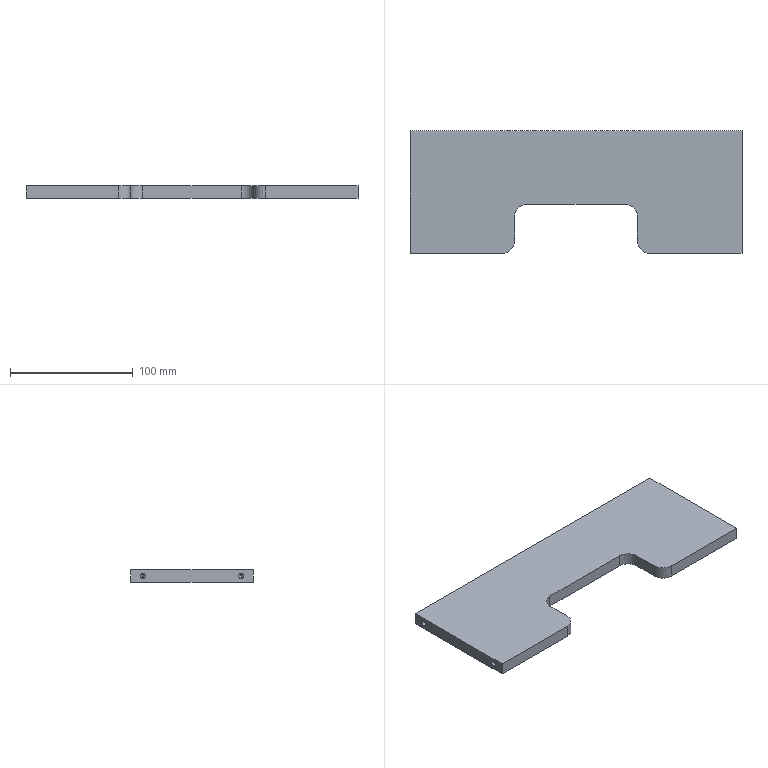Part | STEP file | Grinding bracket middle plate | 1 solid | 30 faces | box 270 x 100 x 10 mm | volume 229012 mm3 | cylinder 12 | plane 10 | cone 8 | commonest cylinder face diameters 4.2 x8 20 x4